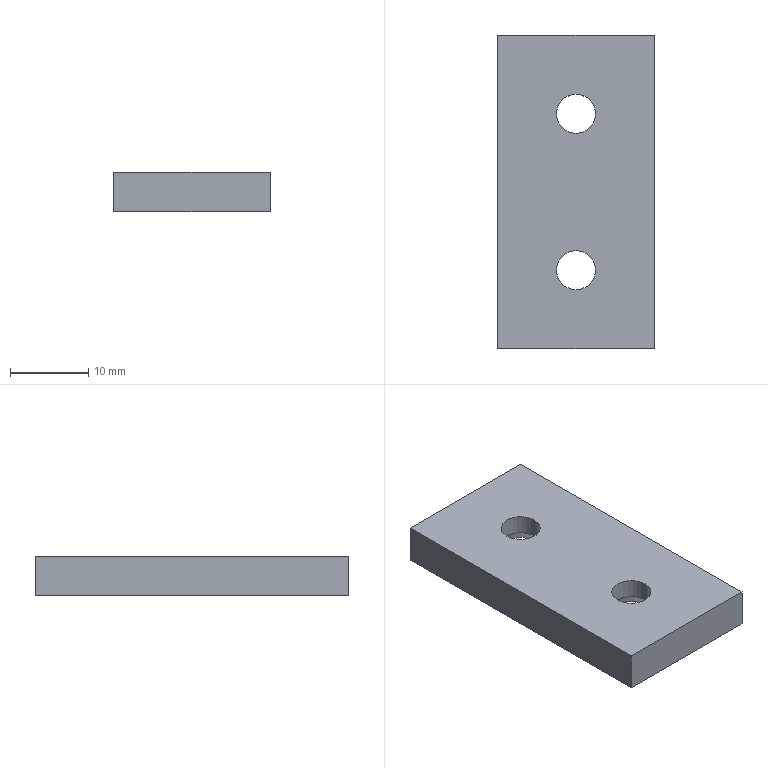Part | SolidWorks | features BaseBody 1 | 1 solid | 14 faces | box 20 x 40 x 5 mm | volume 3673 mm3 | plane 6 | cylinder 4 | cone 4 | commonest cylinder face diameters 5 x4
STEP:
#1=CARTESIAN_POINT('',(86.647,943.5,-366.));
#2=VERTEX_POINT('',#1);
#3=CARTESIAN_POINT('',(91.647,943.5,-366.));
#4=VERTEX_POINT('',#3);
#5=CARTESIAN_POINT('',(89.147,943.5,-366.));
#6=DIRECTION('',(0.,0.,1.));
#7=DIRECTION('',(-1.,0.,0.));
#8=AXIS2_PLACEMENT_3D('',#5,#6,#7);
#9=CIRCLE('',#8,2.5);
#10=EDGE_CURVE('',#2,#4,#9,.T.);
#11=ORIENTED_EDGE('',*,*,#10,.T.);
#12=CARTESIAN_POINT('',(91.647,943.5,-368.5));
#13=VERTEX_POINT('',#12);
#14=CARTESIAN_POINT('',(91.647,943.5,-371.));
#15=DIRECTION('',(0.,0.,-1.));
#16=VECTOR('',#15,1000.);
#17=LINE('',#14,#16);
#18=EDGE_CURVE('',#4,#13,#17,.T.);
#19=ORIENTED_EDGE('',*,*,#18,.T.);
#20=CARTESIAN_POINT('',(86.647,943.5,-368.5));
#21=VERTEX_POINT('',#20);
#22=CARTESIAN_POINT('',(89.147,943.5,-368.5));
#23=DIRECTION('',(0.,0.,1.));
#24=DIRECTION('',(-1.,0.,0.));
#25=AXIS2_PLACEMENT_3D('',#22,#23,#24);
#26=CIRCLE('',#25,2.5);
#27=EDGE_CURVE('',#21,#13,#26,.T.);
#28=ORIENTED_EDGE('',*,*,#27,.F.);
#29=CARTESIAN_POINT('',(86.647,943.5,-371.));
#30=DIRECTION('',(0.,0.,-1.));
#31=VECTOR('',#30,1000.);
#32=LINE('',#29,#31);
#33=EDGE_CURVE('',#2,#21,#32,.T.);
#34=ORIENTED_EDGE('',*,*,#33,.F.);
#35=EDGE_LOOP('',(#11,#19,#28,#34));
#36=FACE_OUTER_BOUND('',#35,.T.);
#37=CARTESIAN_POINT('',(89.147,943.5,-371.));
#38=DIRECTION('',(0.,0.,-1.));
#39=DIRECTION('',(-1.,0.,0.));
#40=AXIS2_PLACEMENT_3D('',#37,#38,#39);
#41=CYLINDRICAL_SURFACE('',#40,2.5);
#42=ADVANCED_FACE('',(#36),#41,.F.);
#43=CARTESIAN_POINT('',(86.647,963.5,-366.));
#44=VERTEX_POINT('',#43);
#45=CARTESIAN_POINT('',(91.647,963.5,-366.));
#46=VERTEX_POINT('',#45);
#47=CARTESIAN_POINT('',(89.147,963.5,-366.));
#48=DIRECTION('',(0.,0.,1.));
#49=DIRECTION('',(-1.,0.,0.));
#50=AXIS2_PLACEMENT_3D('',#47,#48,#49);
#51=CIRCLE('',#50,2.5);
#52=EDGE_CURVE('',#44,#46,#51,.T.);
#53=ORIENTED_EDGE('',*,*,#52,.T.);
#54=CARTESIAN_POINT('',(91.647,963.5,-368.5));
#55=VERTEX_POINT('',#54);
#56=CARTESIAN_POINT('',(91.647,963.5,-371.));
#57=DIRECTION('',(0.,0.,-1.));
#58=VECTOR('',#57,1000.);
#59=LINE('',#56,#58);
#60=EDGE_CURVE('',#46,#55,#59,.T.);
#61=ORIENTED_EDGE('',*,*,#60,.T.);
#62=CARTESIAN_POINT('',(86.647,963.5,-368.5));
#63=VERTEX_POINT('',#62);
#64=CARTESIAN_POINT('',(89.147,963.5,-368.5));
#65=DIRECTION('',(0.,0.,1.));
#66=DIRECTION('',(-1.,0.,0.));
#67=AXIS2_PLACEMENT_3D('',#64,#65,#66);
#68=CIRCLE('',#67,2.5);
#69=EDGE_CURVE('',#63,#55,#68,.T.);
#70=ORIENTED_EDGE('',*,*,#69,.F.);
#71=CARTESIAN_POINT('',(86.647,963.5,-371.));
#72=DIRECTION('',(0.,0.,-1.));
#73=VECTOR('',#72,1000.);
#74=LINE('',#71,#73);
#75=EDGE_CURVE('',#44,#63,#74,.T.);
#76=ORIENTED_EDGE('',*,*,#75,.F.);
#77=EDGE_LOOP('',(#53,#61,#70,#76));
#78=FACE_OUTER_BOUND('',#77,.T.);
#79=CARTESIAN_POINT('',(89.147,963.5,-371.));
#80=DIRECTION('',(0.,0.,-1.));
#81=DIRECTION('',(-1.,0.,0.));
#82=AXIS2_PLACEMENT_3D('',#79,#80,#81);
#83=CYLINDRICAL_SURFACE('',#82,2.5);
#84=ADVANCED_FACE('',(#78),#83,.F.);
#85=ORIENTED_EDGE('',*,*,#27,.T.);
#86=CARTESIAN_POINT('',(94.147,943.5,-371.));
#87=VERTEX_POINT('',#86);
#88=CARTESIAN_POINT('',(94.147,943.5,-371.));
#89=DIRECTION('',(0.7071,0.,-0.7071));
#90=VECTOR('',#89,1000.);
#91=LINE('',#88,#90);
#92=EDGE_CURVE('',#13,#87,#91,.T.);
#93=ORIENTED_EDGE('',*,*,#92,.T.);
#94=CARTESIAN_POINT('',(84.147,943.5,-371.));
#95=VERTEX_POINT('',#94);
#96=CARTESIAN_POINT('',(89.147,943.5,-371.));
#97=DIRECTION('',(0.,0.,1.));
#98=DIRECTION('',(-1.,0.,0.));
#99=AXIS2_PLACEMENT_3D('',#96,#97,#98);
#100=CIRCLE('',#99,5.);
#101=EDGE_CURVE('',#95,#87,#100,.T.);
#102=ORIENTED_EDGE('',*,*,#101,.F.);
#103=CARTESIAN_POINT('',(84.147,943.5,-371.));
#104=DIRECTION('',(-0.7071,0.,-0.7071));
#105=VECTOR('',#104,1000.);
#106=LINE('',#103,#105);
#107=EDGE_CURVE('',#21,#95,#106,.T.);
#108=ORIENTED_EDGE('',*,*,#107,.F.);
#109=EDGE_LOOP('',(#85,#93,#102,#108));
#110=FACE_OUTER_BOUND('',#109,.T.);
#111=CARTESIAN_POINT('',(89.147,943.5,-371.));
#112=DIRECTION('',(0.,0.,-1.));
#113=DIRECTION('',(-1.,0.,0.));
#114=AXIS2_PLACEMENT_3D('',#111,#112,#113);
#115=CONICAL_SURFACE('',#114,5.,0.7854);
#116=ADVANCED_FACE('',(#110),#115,.F.);
#117=ORIENTED_EDGE('',*,*,#69,.T.);
#118=CARTESIAN_POINT('',(94.147,963.5,-371.));
#119=VERTEX_POINT('',#118);
#120=CARTESIAN_POINT('',(94.147,963.5,-371.));
#121=DIRECTION('',(0.7071,0.,-0.7071));
#122=VECTOR('',#121,1000.);
#123=LINE('',#120,#122);
#124=EDGE_CURVE('',#55,#119,#123,.T.);
#125=ORIENTED_EDGE('',*,*,#124,.T.);
#126=CARTESIAN_POINT('',(84.147,963.5,-371.));
#127=VERTEX_POINT('',#126);
#128=CARTESIAN_POINT('',(89.147,963.5,-371.));
#129=DIRECTION('',(0.,0.,1.));
#130=DIRECTION('',(-1.,0.,0.));
#131=AXIS2_PLACEMENT_3D('',#128,#129,#130);
#132=CIRCLE('',#131,5.);
#133=EDGE_CURVE('',#127,#119,#132,.T.);
#134=ORIENTED_EDGE('',*,*,#133,.F.);
#135=CARTESIAN_POINT('',(84.147,963.5,-371.));
#136=DIRECTION('',(-0.7071,0.,-0.7071));
#137=VECTOR('',#136,1000.);
#138=LINE('',#135,#137);
#139=EDGE_CURVE('',#63,#127,#138,.T.);
#140=ORIENTED_EDGE('',*,*,#139,.F.);
#141=EDGE_LOOP('',(#117,#125,#134,#140));
#142=FACE_OUTER_BOUND('',#141,.T.);
#143=CARTESIAN_POINT('',(89.147,963.5,-371.));
#144=DIRECTION('',(0.,0.,-1.));
#145=DIRECTION('',(-1.,0.,0.));
#146=AXIS2_PLACEMENT_3D('',#143,#144,#145);
#147=CONICAL_SURFACE('',#146,5.,0.7854);
#148=ADVANCED_FACE('',(#142),#147,.F.);
#149=ORIENTED_EDGE('',*,*,#10,.F.);
#150=CARTESIAN_POINT('',(89.147,943.5,-366.));
#151=DIRECTION('',(0.,0.,1.));
#152=DIRECTION('',(-1.,0.,0.));
#153=AXIS2_PLACEMENT_3D('',#150,#151,#152);
#154=CIRCLE('',#153,2.5);
#155=EDGE_CURVE('',#4,#2,#154,.T.);
#156=ORIENTED_EDGE('',*,*,#155,.F.);
#157=EDGE_LOOP('',(#149,#156));
#158=FACE_BOUND('',#157,.T.);
#159=ORIENTED_EDGE('',*,*,#52,.F.);
#160=CARTESIAN_POINT('',(89.147,963.5,-366.));
#161=DIRECTION('',(0.,0.,1.));
#162=DIRECTION('',(-1.,0.,0.));
#163=AXIS2_PLACEMENT_3D('',#160,#161,#162);
#164=CIRCLE('',#163,2.5);
#165=EDGE_CURVE('',#46,#44,#164,.T.);
#166=ORIENTED_EDGE('',*,*,#165,.F.);
#167=EDGE_LOOP('',(#159,#166));
#168=FACE_BOUND('',#167,.T.);
#169=CARTESIAN_POINT('',(79.147,973.5,-366.));
#170=VERTEX_POINT('',#169);
#171=CARTESIAN_POINT('',(99.147,973.5,-366.));
#172=VERTEX_POINT('',#171);
#173=CARTESIAN_POINT('',(99.147,973.5,-366.));
#174=DIRECTION('',(1.,0.,0.));
#175=VECTOR('',#174,1000.);
#176=LINE('',#173,#175);
#177=EDGE_CURVE('',#170,#172,#176,.T.);
#178=ORIENTED_EDGE('',*,*,#177,.F.);
#179=CARTESIAN_POINT('',(79.147,933.5,-366.));
#180=VERTEX_POINT('',#179);
#181=CARTESIAN_POINT('',(79.147,933.5,-366.));
#182=DIRECTION('',(0.,1.,0.));
#183=VECTOR('',#182,1000.);
#184=LINE('',#181,#183);
#185=EDGE_CURVE('',#180,#170,#184,.T.);
#186=ORIENTED_EDGE('',*,*,#185,.F.);
#187=CARTESIAN_POINT('',(99.147,933.5,-366.));
#188=VERTEX_POINT('',#187);
#189=CARTESIAN_POINT('',(99.147,933.5,-366.));
#190=DIRECTION('',(-1.,0.,0.));
#191=VECTOR('',#190,1000.);
#192=LINE('',#189,#191);
#193=EDGE_CURVE('',#188,#180,#192,.T.);
#194=ORIENTED_EDGE('',*,*,#193,.F.);
#195=CARTESIAN_POINT('',(99.147,933.5,-366.));
#196=DIRECTION('',(0.,-1.,0.));
#197=VECTOR('',#196,1000.);
#198=LINE('',#195,#197);
#199=EDGE_CURVE('',#172,#188,#198,.T.);
#200=ORIENTED_EDGE('',*,*,#199,.F.);
#201=EDGE_LOOP('',(#178,#186,#194,#200));
#202=FACE_OUTER_BOUND('',#201,.T.);
#203=CARTESIAN_POINT('',(99.147,933.5,-366.));
#204=DIRECTION('',(0.,0.,-1.));
#205=DIRECTION('',(-1.,0.,0.));
#206=AXIS2_PLACEMENT_3D('',#203,#204,#205);
#207=PLANE('',#206);
#208=ADVANCED_FACE('',(#158,#168,#202),#207,.F.);
#209=ORIENTED_EDGE('',*,*,#18,.F.);
#210=ORIENTED_EDGE('',*,*,#155,.T.);
#211=ORIENTED_EDGE('',*,*,#33,.T.);
#212=CARTESIAN_POINT('',(89.147,943.5,-368.5));
#213=DIRECTION('',(0.,0.,1.));
#214=DIRECTION('',(-1.,0.,0.));
#215=AXIS2_PLACEMENT_3D('',#212,#213,#214);
#216=CIRCLE('',#215,2.5);
#217=EDGE_CURVE('',#13,#21,#216,.T.);
#218=ORIENTED_EDGE('',*,*,#217,.F.);
#219=EDGE_LOOP('',(#209,#210,#211,#218));
#220=FACE_OUTER_BOUND('',#219,.T.);
#221=CARTESIAN_POINT('',(89.147,943.5,-371.));
#222=DIRECTION('',(0.,0.,-1.));
#223=DIRECTION('',(-1.,0.,0.));
#224=AXIS2_PLACEMENT_3D('',#221,#222,#223);
#225=CYLINDRICAL_SURFACE('',#224,2.5);
#226=ADVANCED_FACE('',(#220),#225,.F.);
#227=ORIENTED_EDGE('',*,*,#60,.F.);
#228=ORIENTED_EDGE('',*,*,#165,.T.);
#229=ORIENTED_EDGE('',*,*,#75,.T.);
#230=CARTESIAN_POINT('',(89.147,963.5,-368.5));
#231=DIRECTION('',(0.,0.,1.));
#232=DIRECTION('',(-1.,0.,0.));
#233=AXIS2_PLACEMENT_3D('',#230,#231,#232);
#234=CIRCLE('',#233,2.5);
#235=EDGE_CURVE('',#55,#63,#234,.T.);
#236=ORIENTED_EDGE('',*,*,#235,.F.);
#237=EDGE_LOOP('',(#227,#228,#229,#236));
#238=FACE_OUTER_BOUND('',#237,.T.);
#239=CARTESIAN_POINT('',(89.147,963.5,-371.));
#240=DIRECTION('',(0.,0.,-1.));
#241=DIRECTION('',(-1.,0.,0.));
#242=AXIS2_PLACEMENT_3D('',#239,#240,#241);
#243=CYLINDRICAL_SURFACE('',#242,2.5);
#244=ADVANCED_FACE('',(#238),#243,.F.);
#245=CARTESIAN_POINT('',(99.147,973.5,-371.));
#246=VERTEX_POINT('',#245);
#247=CARTESIAN_POINT('',(99.147,933.5,-371.));
#248=VERTEX_POINT('',#247);
#249=CARTESIAN_POINT('',(99.147,933.5,-371.));
#250=DIRECTION('',(0.,-1.,0.));
#251=VECTOR('',#250,1000.);
#252=LINE('',#249,#251);
#253=EDGE_CURVE('',#246,#248,#252,.T.);
#254=ORIENTED_EDGE('',*,*,#253,.F.);
#255=CARTESIAN_POINT('',(99.147,973.5,-371.));
#256=DIRECTION('',(0.,0.,-1.));
#257=VECTOR('',#256,1000.);
#258=LINE('',#255,#257);
#259=EDGE_CURVE('',#172,#246,#258,.T.);
#260=ORIENTED_EDGE('',*,*,#259,.F.);
#261=ORIENTED_EDGE('',*,*,#199,.T.);
#262=CARTESIAN_POINT('',(99.147,933.5,-371.));
#263=DIRECTION('',(0.,0.,1.));
#264=VECTOR('',#263,1000.);
#265=LINE('',#262,#264);
#266=EDGE_CURVE('',#248,#188,#265,.T.);
#267=ORIENTED_EDGE('',*,*,#266,.F.);
#268=EDGE_LOOP('',(#254,#260,#261,#267));
#269=FACE_OUTER_BOUND('',#268,.T.);
#270=CARTESIAN_POINT('',(99.147,933.5,-371.));
#271=DIRECTION('',(-1.,0.,0.));
#272=DIRECTION('',(0.,0.,1.));
#273=AXIS2_PLACEMENT_3D('',#270,#271,#272);
#274=PLANE('',#273);
#275=ADVANCED_FACE('',(#269),#274,.F.);
#276=CARTESIAN_POINT('',(79.147,973.5,-371.));
#277=VERTEX_POINT('',#276);
#278=CARTESIAN_POINT('',(99.147,973.5,-371.));
#279=DIRECTION('',(1.,0.,0.));
#280=VECTOR('',#279,1000.);
#281=LINE('',#278,#280);
#282=EDGE_CURVE('',#277,#246,#281,.T.);
#283=ORIENTED_EDGE('',*,*,#282,.F.);
#284=CARTESIAN_POINT('',(79.147,973.5,-371.));
#285=DIRECTION('',(0.,0.,-1.));
#286=VECTOR('',#285,1000.);
#287=LINE('',#284,#286);
#288=EDGE_CURVE('',#170,#277,#287,.T.);
#289=ORIENTED_EDGE('',*,*,#288,.F.);
#290=ORIENTED_EDGE('',*,*,#177,.T.);
#291=ORIENTED_EDGE('',*,*,#259,.T.);
#292=EDGE_LOOP('',(#283,#289,#290,#291));
#293=FACE_OUTER_BOUND('',#292,.T.);
#294=CARTESIAN_POINT('',(99.147,973.5,-371.));
#295=DIRECTION('',(0.,-1.,0.));
#296=DIRECTION('',(0.,0.,-1.));
#297=AXIS2_PLACEMENT_3D('',#294,#295,#296);
#298=PLANE('',#297);
#299=ADVANCED_FACE('',(#293),#298,.F.);
#300=CARTESIAN_POINT('',(79.147,933.5,-371.));
#301=VERTEX_POINT('',#300);
#302=CARTESIAN_POINT('',(79.147,933.5,-371.));
#303=DIRECTION('',(0.,1.,0.));
#304=VECTOR('',#303,1000.);
#305=LINE('',#302,#304);
#306=EDGE_CURVE('',#301,#277,#305,.T.);
#307=ORIENTED_EDGE('',*,*,#306,.F.);
#308=CARTESIAN_POINT('',(79.147,933.5,-371.));
#309=DIRECTION('',(0.,0.,-1.));
#310=VECTOR('',#309,1000.);
#311=LINE('',#308,#310);
#312=EDGE_CURVE('',#180,#301,#311,.T.);
#313=ORIENTED_EDGE('',*,*,#312,.F.);
#314=ORIENTED_EDGE('',*,*,#185,.T.);
#315=ORIENTED_EDGE('',*,*,#288,.T.);
#316=EDGE_LOOP('',(#307,#313,#314,#315));
#317=FACE_OUTER_BOUND('',#316,.T.);
#318=CARTESIAN_POINT('',(79.147,933.5,-371.));
#319=DIRECTION('',(1.,0.,0.));
#320=DIRECTION('',(0.,0.,-1.));
#321=AXIS2_PLACEMENT_3D('',#318,#319,#320);
#322=PLANE('',#321);
#323=ADVANCED_FACE('',(#317),#322,.F.);
#324=CARTESIAN_POINT('',(99.147,933.5,-371.));
#325=DIRECTION('',(-1.,0.,0.));
#326=VECTOR('',#325,1000.);
#327=LINE('',#324,#326);
#328=EDGE_CURVE('',#248,#301,#327,.T.);
#329=ORIENTED_EDGE('',*,*,#328,.F.);
#330=ORIENTED_EDGE('',*,*,#266,.T.);
#331=ORIENTED_EDGE('',*,*,#193,.T.);
#332=ORIENTED_EDGE('',*,*,#312,.T.);
#333=EDGE_LOOP('',(#329,#330,#331,#332));
#334=FACE_OUTER_BOUND('',#333,.T.);
#335=CARTESIAN_POINT('',(99.147,933.5,-371.));
#336=DIRECTION('',(0.,1.,0.));
#337=DIRECTION('',(0.,0.,1.));
#338=AXIS2_PLACEMENT_3D('',#335,#336,#337);
#339=PLANE('',#338);
#340=ADVANCED_FACE('',(#334),#339,.F.);
#341=ORIENTED_EDGE('',*,*,#92,.F.);
#342=ORIENTED_EDGE('',*,*,#217,.T.);
#343=ORIENTED_EDGE('',*,*,#107,.T.);
#344=CARTESIAN_POINT('',(89.147,943.5,-371.));
#345=DIRECTION('',(0.,0.,1.));
#346=DIRECTION('',(-1.,0.,0.));
#347=AXIS2_PLACEMENT_3D('',#344,#345,#346);
#348=CIRCLE('',#347,5.);
#349=EDGE_CURVE('',#87,#95,#348,.T.);
#350=ORIENTED_EDGE('',*,*,#349,.F.);
#351=EDGE_LOOP('',(#341,#342,#343,#350));
#352=FACE_OUTER_BOUND('',#351,.T.);
#353=CARTESIAN_POINT('',(89.147,943.5,-371.));
#354=DIRECTION('',(0.,0.,-1.));
#355=DIRECTION('',(-1.,0.,0.));
#356=AXIS2_PLACEMENT_3D('',#353,#354,#355);
#357=CONICAL_SURFACE('',#356,5.,0.7854);
#358=ADVANCED_FACE('',(#352),#357,.F.);
#359=ORIENTED_EDGE('',*,*,#124,.F.);
#360=ORIENTED_EDGE('',*,*,#235,.T.);
#361=ORIENTED_EDGE('',*,*,#139,.T.);
#362=CARTESIAN_POINT('',(89.147,963.5,-371.));
#363=DIRECTION('',(0.,0.,1.));
#364=DIRECTION('',(-1.,0.,0.));
#365=AXIS2_PLACEMENT_3D('',#362,#363,#364);
#366=CIRCLE('',#365,5.);
#367=EDGE_CURVE('',#119,#127,#366,.T.);
#368=ORIENTED_EDGE('',*,*,#367,.F.);
#369=EDGE_LOOP('',(#359,#360,#361,#368));
#370=FACE_OUTER_BOUND('',#369,.T.);
#371=CARTESIAN_POINT('',(89.147,963.5,-371.));
#372=DIRECTION('',(0.,0.,-1.));
#373=DIRECTION('',(-1.,0.,0.));
#374=AXIS2_PLACEMENT_3D('',#371,#372,#373);
#375=CONICAL_SURFACE('',#374,5.,0.7854);
#376=ADVANCED_FACE('',(#370),#375,.F.);
#377=ORIENTED_EDGE('',*,*,#101,.T.);
#378=ORIENTED_EDGE('',*,*,#349,.T.);
#379=EDGE_LOOP('',(#377,#378));
#380=FACE_BOUND('',#379,.T.);
#381=ORIENTED_EDGE('',*,*,#133,.T.);
#382=ORIENTED_EDGE('',*,*,#367,.T.);
#383=EDGE_LOOP('',(#381,#382));
#384=FACE_BOUND('',#383,.T.);
#385=ORIENTED_EDGE('',*,*,#253,.T.);
#386=ORIENTED_EDGE('',*,*,#328,.T.);
#387=ORIENTED_EDGE('',*,*,#306,.T.);
#388=ORIENTED_EDGE('',*,*,#282,.T.);
#389=EDGE_LOOP('',(#385,#386,#387,#388));
#390=FACE_OUTER_BOUND('',#389,.T.);
#391=CARTESIAN_POINT('',(99.147,933.5,-371.));
#392=DIRECTION('',(0.,0.,-1.));
#393=DIRECTION('',(-1.,0.,0.));
#394=AXIS2_PLACEMENT_3D('',#391,#392,#393);
#395=PLANE('',#394);
#396=ADVANCED_FACE('',(#380,#384,#390),#395,.T.);
#397=CLOSED_SHELL('',(#42,#84,#116,#148,#208,#226,#244,#275,#299,#323,#340,#358,#376,#396));
#398=MANIFOLD_SOLID_BREP('',#397);
#399=CARTESIAN_POINT('',(0.,0.,0.));
#400=DIRECTION('',(0.,0.,1.));
#401=DIRECTION('',(1.,0.,0.));
#402=AXIS2_PLACEMENT_3D('',#399,#400,#401);
#403=(LENGTH_UNIT()NAMED_UNIT(*)SI_UNIT(.MILLI.,.METRE.));
#404=UNCERTAINTY_MEASURE_WITH_UNIT(LENGTH_MEASURE(0.00001),#403,'','');
#405=(NAMED_UNIT(*)PLANE_ANGLE_UNIT()SI_UNIT($,.RADIAN.));
#406=(NAMED_UNIT(*)SI_UNIT($,.STERADIAN.)SOLID_ANGLE_UNIT());
#407=(GEOMETRIC_REPRESENTATION_CONTEXT(3)GLOBAL_UNCERTAINTY_ASSIGNED_CONTEXT((#404))GLOBAL_UNIT_ASSIGNED_CONTEXT((#403,#405,#406))REPRESENTATION_CONTEXT('',''));
#408=ADVANCED_BREP_SHAPE_REPRESENTATION('',(#398,#402),#407);